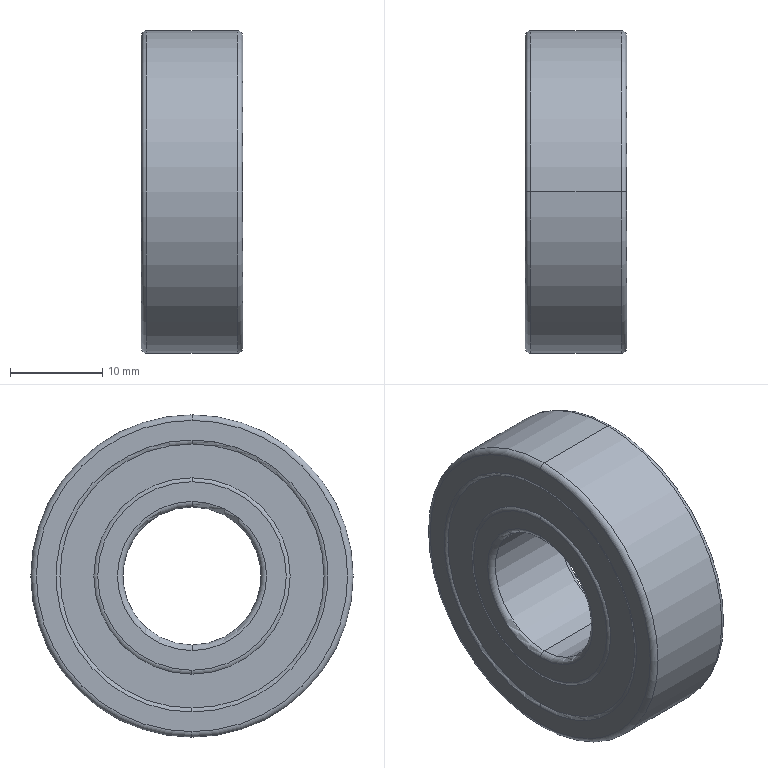Part | SolidWorks | features Revolution 5, CirPattern 2, RefAxis 1, RevCut 1 | 15 solids | 178 faces | box 11 x 35 x 35 mm | volume 6580 mm3 | cylinder 62 | sphere 56 | plane 34 | torus 26 | commonest cylinder face diameters 24 x25 26 x25 21.667 x4 28.333 x4 15 x2 35 x2